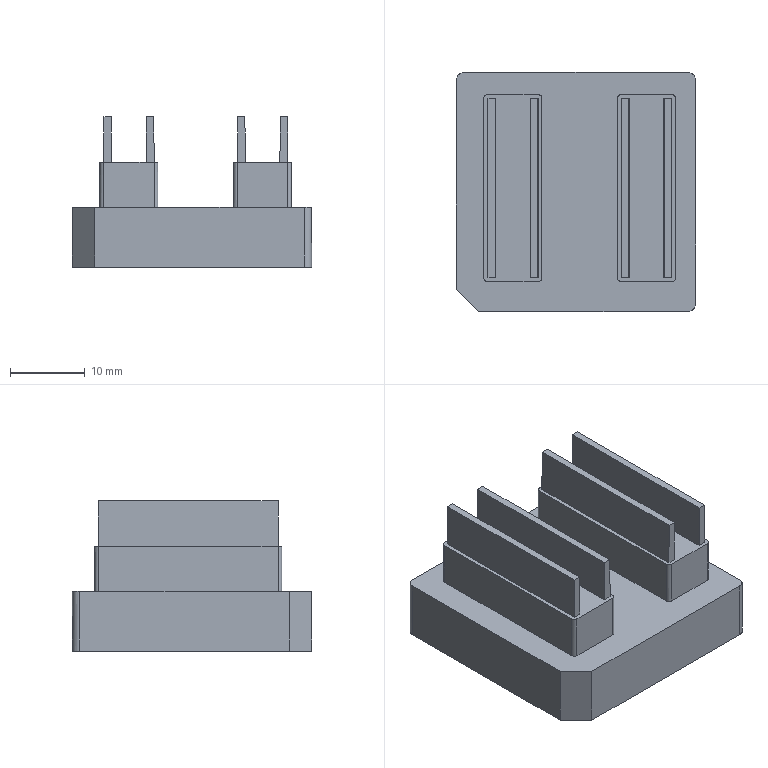NC program | PowerMill | posted with a generic post | part box 32 x 32 x 20.109 mm
Lines 18577 to 19554 of 124326:
N18674 M6
N18675 S18000 M03
N18676 G00 G90 X0.0 Y0.0
N18677 G43 Z10.799 H10
N18678
N18679 G05 P10000 R8
N18680 X9.9087 Y3.019
N18681 Z0.909
N18682 G01 Z-0.291 F1200.0
N18683 X9.9524 Y3.021 F2000.0
N18684 X9.9957 Y3.0269
N18685 X10.0383 Y3.0368
N18686 X10.0799 Y3.0506
N18687 X10.12 Y3.068
N18688 X10.1584 Y3.0891
N18689 X10.1947 Y3.1135
N18690 X10.2286 Y3.1412
N18691 X10.2599 Y3.1718
N18692 X10.2882 Y3.2051
N18693 X10.3134 Y3.2409
N18694 X10.3352 Y3.2788
N18695 X10.3535 Y3.3186
N18696 X10.3681 Y3.3599
N18697 X10.3788 Y3.4023
N18698 X10.3857 Y3.4455
N18699 X10.3886 Y3.4891
N18700 X10.3887 Y3.499
N18701 Y9.4972
N18702 X10.3886 Y11.6966
N18703 X10.3881 Y12.4964
N18704 X10.39 Y12.5743
N18705 X10.3958 Y12.6519
N18706 X10.4056 Y12.7286
N18707 X10.4192 Y12.8042
N18708 X10.4365 Y12.8783
N18709 X10.4575 Y12.9506
N18710 X10.482 Y13.0208
N18711 X10.5098 Y13.0888
N18712 X10.5412 Y13.1551
N18713 X10.5769 Y13.2214
N18714 X10.616 Y13.2858
N18715 X10.6586 Y13.3481
N18716 X10.7044 Y13.408
N18717 X10.7533 Y13.4655
N18718 X10.8052 Y13.5203
N18719 X10.8599 Y13.5723
N18720 X10.9172 Y13.6212
N18721 X10.9769 Y13.667
N18722 X11.039 Y13.7095
N18723 X11.1032 Y13.7487
N18724 X11.1695 Y13.7845
N18725 X11.2373 Y13.8166
N18726 X11.3079 Y13.8456
N18727 X11.3794 Y13.8707
N18728 X11.4516 Y13.8919
N18729 X11.5242 Y13.9091
N18730 X11.5972 Y13.9222
N18731 X11.6701 Y13.9314
N18732 X11.7429 Y13.9366
N18733 X11.8156 Y13.9379
N18734 X12.5481 Y13.9385
N18735 X12.7962 Y13.9378
N18736 X12.8681 Y13.9356
N18737 X12.9404 Y13.9294
N18738 X13.0129 Y13.9191
N18739 X13.0856 Y13.9048
N18740 X13.1581 Y13.8865
N18741 X13.2303 Y13.8642
N18742 X13.3019 Y13.8379
N18743 X13.3726 Y13.8077
N18744 X13.4395 Y13.7749
N18745 X13.5046 Y13.7386
N18746 X13.568 Y13.6987
N18747 X13.6293 Y13.6554
N18748 X13.6884 Y13.6087
N18749 X13.7452 Y13.5589
N18750 X13.7987 Y13.5066
N18751 X13.8494 Y13.4516
N18752 X13.8973 Y13.3938
N18753 X13.9422 Y13.3333
N18754 X13.984 Y13.2702
N18755 X14.0227 Y13.2048
N18756 X14.058 Y13.137
N18757 X14.0899 Y13.0672
N18758 X14.1164 Y13.0003
N18759 X14.1393 Y12.9316
N18760 X14.1588 Y12.8606
N18761 X14.1748 Y12.7875
N18762 X14.1872 Y12.7125
N18763 X14.1958 Y12.6355
N18764 X14.2007 Y12.5567
N18765 X14.2018 Y12.4763
N18766 Y-1.4479
N18767 Y-9.9971
N18768 X14.2017 Y-11.0461
N18769 X14.2022 Y-11.4967
N18770 X14.2004 Y-11.5753
N18771 X14.1946 Y-11.6529
N18772 X14.1851 Y-11.7293
N18773 X14.1717 Y-11.804
N18774 X14.1547 Y-11.8769
N18775 X14.1341 Y-11.9478
N18776 X14.1101 Y-12.0169
N18777 X14.0815 Y-12.0865
N18778 X14.0494 Y-12.1546
N18779 X14.0137 Y-12.221
N18780 X13.9746 Y-12.2853
N18781 X13.9321 Y-12.3476
N18782 X13.8863 Y-12.4076
N18783 X13.8374 Y-12.4651
N18784 X13.7855 Y-12.5199
N18785 X13.7308 Y-12.5719
N18786 X13.6734 Y-12.621
N18787 X13.6136 Y-12.6668
N18788 X13.5515 Y-12.7094
N18789 X13.4873 Y-12.7487
N18790 X13.4211 Y-12.7844
N18791 X13.3532 Y-12.8166
N18792 X13.2838 Y-12.8452
N18793 X13.213 Y-12.87
N18794 X13.1409 Y-12.8911
N18795 X13.1212 Y-12.8961
N18796 X13.047 Y-12.9127
N18797 X12.9737 Y-12.925
N18798 X12.9016 Y-12.9332
N18799 X12.8308 Y-12.9375
N18800 X12.7606 Y-12.9382
N18801 X12.2312 Y-12.9385
N18802 X11.7966 Y-12.9378
N18803 X11.724 Y-12.9358
N18804 X11.6514 Y-12.9297
N18805 X11.5788 Y-12.9197
N18806 X11.5064 Y-12.9057
N18807 X11.4343 Y-12.8877
N18808 X11.3628 Y-12.8657
N18809 X11.2921 Y-12.8398
N18810 X11.2224 Y-12.81
N18811 X11.154 Y-12.7764
N18812 X11.0871 Y-12.7391
N18813 X11.0219 Y-12.6983
N18814 X10.962 Y-12.6561
N18815 X10.9038 Y-12.6103
N18816 X10.8474 Y-12.5609
N18817 X10.7935 Y-12.5085
N18818 X10.7425 Y-12.4533
N18819 X10.6944 Y-12.3954
N18820 X10.6494 Y-12.335
N18821 X10.6075 Y-12.2721
N18822 X10.5689 Y-12.207
N18823 X10.5337 Y-12.1397
N18824 X10.502 Y-12.0705
N18825 X10.4739 Y-11.9996
N18826 X10.451 Y-11.9314
N18827 X10.4316 Y-11.8612
N18828 X10.4157 Y-11.7888
N18829 X10.4034 Y-11.7142
N18830 X10.3947 Y-11.6375
N18831 X10.3898 Y-11.5587
N18832 X10.3887 Y-11.4781
N18833 Y3.499
N18834 X10.3867 Y3.5427
N18835 X10.3807 Y3.586
N18836 X10.3708 Y3.6287
N18837 X10.3571 Y3.6702
N18838 X10.3396 Y3.7104
N18839 X10.3186 Y3.7487
N18840 X10.2941 Y3.785
N18841 X10.2665 Y3.8189
N18842 X10.2359 Y3.8502
N18843 X10.2025 Y3.8785
N18844 X10.1668 Y3.9037
N18845 X10.1288 Y3.9255
N18846 X10.089 Y3.9438
N18847 X10.0478 Y3.9584
N18848 X10.0054 Y3.9691
N18849 X9.9622 Y3.976
N18850 X9.9185 Y3.9789
N18851 X9.9087 Y3.979
N18852 X9.9083 Y3.019 Z-0.331
N18853 X9.952 Y3.021
N18854 X9.9953 Y3.0269
N18855 X10.038 Y3.0368
N18856 X10.0795 Y3.0506
N18857 X10.1197 Y3.068
N18858 X10.158 Y3.0891
N18859 X10.1943 Y3.1135
N18860 X10.2282 Y3.1412
N18861 X10.2595 Y3.1718
N18862 X10.2878 Y3.2051
N18863 X10.313 Y3.2409
N18864 X10.3348 Y3.2788
N18865 X10.3531 Y3.3186
N18866 X10.3677 Y3.3599
N18867 X10.3784 Y3.4023
N18868 X10.3853 Y3.4455
N18869 X10.3882 Y3.4891
N18870 X10.3883 Y3.499
N18871 Y10.9968
N18872 Y12.4963
N18873 X10.3902 Y12.5756
N18874 X10.396 Y12.6536
N18875 X10.4057 Y12.7303
N18876 X10.4191 Y12.8053
N18877 X10.4362 Y12.8786
N18878 X10.4569 Y12.9499
N18879 X10.481 Y13.0192
N18880 X10.5087 Y13.0866
N18881 X10.541 Y13.1551
N18882 X10.577 Y13.2218
N18883 X10.6163 Y13.2865
N18884 X10.659 Y13.349
N18885 X10.7049 Y13.409
N18886 X10.7538 Y13.4664
N18887 X10.8056 Y13.5211
N18888 X10.8601 Y13.5729
N18889 X10.9173 Y13.6217
N18890 X10.9769 Y13.6674
N18891 X11.0388 Y13.7097
N18892 X11.1033 Y13.7491
N18893 X11.1698 Y13.785
N18894 X11.238 Y13.8173
N18895 X11.3078 Y13.8459
N18896 X11.3788 Y13.8708
N18897 X11.451 Y13.8918
N18898 X11.524 Y13.9089
N18899 X11.5976 Y13.9221
N18900 X11.6718 Y13.9313
N18901 X11.7463 Y13.9365
N18902 X11.821 Y13.938
N18903 X12.1312 Y13.9386
N18904 X12.665 Y13.9382
N18905 X12.7963 Y13.9378
N18906 X12.8692 Y13.9355
N18907 X12.9421 Y13.9292
N18908 X13.0151 Y13.9189
N18909 X13.0878 Y13.9046
N18910 X13.1602 Y13.8864
N18911 X13.232 Y13.8642
N18912 X13.303 Y13.838
N18913 X13.373 Y13.808
N18914 X13.4403 Y13.7748
N18915 X13.5058 Y13.7381
N18916 X13.5694 Y13.698
N18917 X13.6309 Y13.6544
N18918 X13.69 Y13.6076
N18919 X13.7468 Y13.5576
N18920 X13.8008 Y13.5047
N18921 X13.8521 Y13.4489
N18922 X13.8991 Y13.392
N18923 X13.9431 Y13.3327
N18924 X13.9843 Y13.2705
N18925 X14.0226 Y13.2055
N18926 X14.058 Y13.1377
N18927 X14.0902 Y13.0671
N18928 X14.1167 Y13.0006
N18929 X14.1396 Y12.9322
N18930 X14.159 Y12.8615
N18931 X14.175 Y12.7887
N18932 X14.1874 Y12.7138
N18933 X14.1961 Y12.6369
N18934 X14.201 Y12.5581
N18935 X14.2021 Y12.4776
N18936 Y-1.9367
N18937 Y-9.9971
N18938 Y-11.4966
N18939 X14.2002 Y-11.5768
N18940 X14.1945 Y-11.655
N18941 X14.185 Y-11.7311
N18942 X14.1719 Y-11.8051
N18943 X14.1552 Y-11.8768
N18944 X14.1351 Y-11.9463
N18945 X14.1114 Y-12.014
N18946 X14.0823 Y-12.0853
N18947 X14.0498 Y-12.1543
N18948 X14.0141 Y-12.2209
N18949 X13.9753 Y-12.285
N18950 X13.9335 Y-12.3464
N18951 X13.8886 Y-12.4052
N18952 X13.8396 Y-12.4629
N18953 X13.7876 Y-12.518
N18954 X13.7329 Y-12.5702
N18955 X13.6755 Y-12.6194
N18956 X13.6156 Y-12.6655
N18957 X13.5535 Y-12.7083
N18958 X13.4892 Y-12.7476
N18959 X13.4231 Y-12.7835
N18960 X13.3552 Y-12.8158
N18961 X13.2858 Y-12.8444
N18962 X13.215 Y-12.8693
N18963 X13.143 Y-12.8904
N18964 X13.1215 Y-12.8958
N18965 X13.1212 Y-12.8959
N18966 X13.0454 Y-12.9128
N18967 X12.9721 Y-12.9252
N18968 X12.9015 Y-12.9335
N18969 X12.8332 Y-12.9376
N18970 X12.7662 Y-12.9383
N18971 X12.2196 Y-12.9387
N18972 X11.7966 Y-12.938
N18973 X11.7238 Y-12.9357
N18974 X11.6508 Y-12.9294
N18975 X11.5777 Y-12.9191
N18976 X11.5047 Y-12.9049
N18977 X11.432 Y-12.8866
N18978 X11.3598 Y-12.8643
N18979 X11.2884 Y-12.8381
N18980 X11.2181 Y-12.8081
N18981 X11.151 Y-12.7752
N18982 X11.0856 Y-12.7388
N18983 X11.0222 Y-12.6988
N18984 X10.9608 Y-12.6554
N18985 X10.9016 Y-12.6088
N18986 X10.8449 Y-12.5589
N18987 X10.7912 Y-12.5065
N18988 X10.7404 Y-12.4512
N18989 X10.6924 Y-12.3933
N18990 X10.6474 Y-12.3327
N18991 X10.6056 Y-12.2695
N18992 X10.5669 Y-12.204
N18993 X10.5315 Y-12.1362
N18994 X10.5011 Y-12.0699
N18995 X10.4744 Y-12.0022
N18996 X10.4511 Y-11.9326
N18997 X10.4315 Y-11.8611
N18998 X10.4154 Y-11.7878
N18999 X10.403 Y-11.7126
N19000 X10.3943 Y-11.6357
N19001 X10.3894 Y-11.5571
N19002 X10.3883 Y-11.477
N19003 Y1.9985
N19004 Y3.499
N19005 X10.3863 Y3.5427
N19006 X10.3803 Y3.586
N19007 X10.3704 Y3.6287
N19008 X10.3567 Y3.6702
N19009 X10.3392 Y3.7104
N19010 X10.3182 Y3.7487
N19011 X10.2937 Y3.785
N19012 X10.2661 Y3.8189
N19013 X10.2355 Y3.8502
N19014 X10.2021 Y3.8785
N19015 X10.1664 Y3.9037
N19016 X10.1284 Y3.9255
N19017 X10.0887 Y3.9438
N19018 X10.0474 Y3.9584
N19019 X10.005 Y3.9691
N19020 X9.9618 Y3.976
N19021 X9.9181 Y3.9789
N19022 X9.9083 Y3.979
N19023 X9.9079 Y3.019 Z-0.371
N19024 X9.9516 Y3.021
N19025 X9.995 Y3.0269
N19026 X10.0376 Y3.0368
N19027 X10.0792 Y3.0506
N19028 X10.1193 Y3.068
N19029 X10.1577 Y3.0891
N19030 X10.194 Y3.1135
N19031 X10.2279 Y3.1412
N19032 X10.2591 Y3.1718
N19033 X10.2875 Y3.2051
N19034 X10.3126 Y3.2409
N19035 X10.3345 Y3.2788
N19036 X10.3527 Y3.3186
N19037 X10.3673 Y3.3599
N19038 X10.3781 Y3.4023
N19039 X10.3849 Y3.4455
N19040 X10.3878 Y3.4891
N19041 X10.3879 Y3.499
N19042 Y5.089
N19043 Y12.4963
N19044 X10.3896 Y12.5773
N19045 X10.3946 Y12.6507
N19046 X10.403 Y12.7203
N19047 X10.4159 Y12.7945
N19048 X10.4327 Y12.8679
N19049 X10.4534 Y12.9404
N19050 X10.4779 Y13.0117
N19051 X10.5061 Y13.0817
N19052 X10.538 Y13.1501
N19053 X10.5735 Y13.2167
N19054 X10.6124 Y13.2813
N19055 X10.6547 Y13.3437
N19056 X10.7002 Y13.4038
N19057 X10.7488 Y13.4613
N19058 X10.8003 Y13.5162
N19059 X10.8547 Y13.5683
N19060 X10.9117 Y13.6173
N19061 X10.9715 Y13.6636
N19062 X11.0331 Y13.7062
N19063 X11.0962 Y13.7452
N19064 X11.1608 Y13.7804
N19065 X11.2269 Y13.812
N19066 X11.2988 Y13.842
N19067 X11.3711 Y13.868
N19068 X11.4437 Y13.8899
N19069 X11.5161 Y13.9077
N19070 X11.5884 Y13.9214
N19071 X11.6602 Y13.9311
N19072 X11.7315 Y13.9367
N19073 X11.8023 Y13.9384
N19074 X12.2964
N19075 X12.662
N19076 X12.7963 Y13.9378
N19077 X12.8703 Y13.9352
N19078 X12.9442 Y13.9287
N19079 X13.0179 Y13.9182
N19080 X13.0912 Y13.9037
N19081 X13.1638 Y13.8852
N19082 X13.2357 Y13.8629
N19083 X13.3066 Y13.8367
N19084 X13.3762 Y13.8066
N19085 X13.4434 Y13.7734
N19086 X13.5089 Y13.7365
N19087 X13.5724 Y13.6962
N19088 X13.6339 Y13.6524
N19089 X13.6931 Y13.6054
N19090 X13.7498 Y13.5551
N19091 X13.803 Y13.5029
N19092 X13.8534 Y13.4479
N19093 X13.9009 Y13.3901
N19094 X13.9455 Y13.3296
N19095 X13.9872 Y13.2664
N19096 X14.0257 Y13.2007
N19097 X14.0609 Y13.1326
N19098 X14.0911 Y13.0663
N19099 X14.1177 Y12.9985
N19100 X14.1407 Y12.929
N19101 X14.1602 Y12.8574
N19102 X14.1761 Y12.784
N19103 X14.1883 Y12.7088
N19104 X14.1968 Y12.6318
N19105 X14.2015 Y12.5531
N19106 X14.2025 Y12.4728
N19107 Y-0.872
N19108 Y-8.6378
N19109 X14.2026 Y-10.7936
N19110 X14.2028 Y-11.4966
N19111 X14.2009 Y-11.5762
N19112 X14.1952 Y-11.6541
N19113 X14.1857 Y-11.7302
N19114 X14.1725 Y-11.8043
N19115 X14.1557 Y-11.8763
N19116 X14.1354 Y-11.9462
N19117 X14.1116 Y-12.0143
N19118 X14.0823 Y-12.0858
N19119 X14.0499 Y-12.1549
N19120 X14.0144 Y-12.2212
N19121 X13.9758 Y-12.2849
N19122 X13.9345 Y-12.3456
N19123 X13.8902 Y-12.4036
N19124 X13.8402 Y-12.4626
N19125 X13.7886 Y-12.5176
N19126 X13.7352 Y-12.5687
N19127 X13.6796 Y-12.6167
N19128 X13.6197 Y-12.663
N19129 X13.5576 Y-12.706
N19130 X13.4935 Y-12.7456
N19131 X13.4274 Y-12.7817
N19132 X13.3597 Y-12.8142
N19133 X13.2904 Y-12.8429
N19134 X13.2197 Y-12.868
N19135 X13.1478 Y-12.8892
N19136 X13.1219 Y-12.8959
N19137 X13.1212 Y-12.896
N19138 X13.0456 Y-12.9128
N19139 X12.9721 Y-12.9253
N19140 X12.9014 Y-12.9335
N19141 X12.8331 Y-12.9376
N19142 X12.766 Y-12.9383
N19143 X12.2057 Y-12.9387
N19144 X11.7966 Y-12.9379
N19145 X11.7236 Y-12.9357
N19146 X11.6505 Y-12.9294
N19147 X11.5773 Y-12.9191
N19148 X11.5043 Y-12.9048
N19149 X11.4316 Y-12.8866
N19150 X11.3595 Y-12.8644
N19151 X11.2882 Y-12.8382
N19152 X11.218 Y-12.8082
N19153 X11.1506 Y-12.7752
N19154 X11.0851 Y-12.7386
N19155 X11.0215 Y-12.6986
N19156 X10.9601 Y-12.6552
N19157 X10.9009 Y-12.6085
N19158 X10.8443 Y-12.5587
N19159 X10.7903 Y-12.506
N19160 X10.7393 Y-12.4505
N19161 X10.6915 Y-12.3927
N19162 X10.6469 Y-12.3325
N19163 X10.6053 Y-12.2699
N19164 X10.567 Y-12.2048
N19165 X10.5319 Y-12.1373
N19166 X10.5001 Y-12.0677
N19167 X10.472 Y-11.9965
N19168 X10.4494 Y-11.9288
N19169 X10.4302 Y-11.859
N19170 X10.4145 Y-11.7868
N19171 X10.4023 Y-11.7124
N19172 X10.3938 Y-11.6357
N19173 X10.389 Y-11.5569
N19174 X10.3879 Y-11.476
N19175 Y3.499
N19176 X10.3859 Y3.5427
N19177 X10.38 Y3.586
N19178 X10.3701 Y3.6287
N19179 X10.3563 Y3.6702
N19180 X10.3389 Y3.7104
N19181 X10.3178 Y3.7487
N19182 X10.2934 Y3.785
N19183 X10.2657 Y3.8189
N19184 X10.2351 Y3.8502
N19185 X10.2018 Y3.8785
N19186 X10.166 Y3.9037
N19187 X10.1281 Y3.9255
N19188 X10.0883 Y3.9438
N19189 X10.0471 Y3.9584
N19190 X10.0046 Y3.9691
N19191 X9.9614 Y3.976
N19192 X9.9178 Y3.9789
N19193 X9.9079 Y3.979
N19194 X9.9076 Y3.019 Z-0.411
N19195 X9.9513 Y3.021
N19196 X9.9946 Y3.0269
N19197 X10.0373 Y3.0368
N19198 X10.0788 Y3.0506
N19199 X10.119 Y3.068
N19200 X10.1573 Y3.0891
N19201 X10.1936 Y3.1135
N19202 X10.2275 Y3.1412
N19203 X10.2588 Y3.1718
N19204 X10.2871 Y3.2051
N19205 X10.3123 Y3.2409
N19206 X10.3341 Y3.2788
N19207 X10.3524 Y3.3186
N19208 X10.367 Y3.3599
N19209 X10.3777 Y3.4023
N19210 X10.3846 Y3.4455
N19211 X10.3875 Y3.4891
N19212 X10.3876 Y3.499
N19213 Y5.1533
N19214 Y12.4963
N19215 X10.3893 Y12.5773
N19216 X10.3943 Y12.6512
N19217 X10.4028 Y12.7213
N19218 X10.4158 Y12.7956
N19219 X10.4326 Y12.8691
N19220 X10.4534 Y12.9415
N19221 X10.4779 Y13.0128
N19222 X10.5062 Y13.0827
N19223 X10.5381 Y13.1511
N19224 X10.5737 Y13.2176
N19225 X10.6127 Y13.2822
N19226 X10.655 Y13.3446
N19227 X10.7006 Y13.4046
N19228 X10.7493 Y13.4622
N19229 X10.8009 Y13.5171
N19230 X10.8554 Y13.5691
N19231 X10.9124 Y13.6181
N19232 X10.9723 Y13.6643
N19233 X11.0345 Y13.7072
N19234 X11.0989 Y13.7468
N19235 X11.1652 Y13.783
N19236 X11.2333 Y13.8155
N19237 X11.3029 Y13.8444
N19238 X11.3738 Y13.8694
N19239 X11.4457 Y13.8907
N19240 X11.5185 Y13.908
N19241 X11.5919 Y13.9214
N19242 X11.6658 Y13.9308
N19243 X11.74 Y13.9363
N19244 X11.8144 Y13.9378
N19245 X12.2538 Y13.9388
N19246 X12.6931 Y13.9381
N19247 X12.7959 Y13.938
N19248 X12.8664 Y13.936
N19249 X12.9379 Y13.93
N19250 X13.0102 Y13.9199
N19251 X13.083 Y13.9058
N19252 X13.1558 Y13.8875
N19253 X13.2284 Y13.8653
N19254 X13.3001 Y13.8392
N19255 X13.3706 Y13.8093
N19256 X13.4369 Y13.777
N19257 X13.5017 Y13.7411
N19258 X13.5651 Y13.7013
N19259 X13.6267 Y13.658
N19260 X13.6863 Y13.6113
N19261 X13.7434 Y13.5614
N19262 X13.7978 Y13.5086
N19263 X13.8491 Y13.4531
N19264 X13.8973 Y13.3954
N19265 X13.942 Y13.3355
N19266 X13.9832 Y13.2737
N19267 X14.0213 Y13.2095
N19268 X14.0563 Y13.1424
N19269 X14.0884 Y13.0727
N19270 X14.1172 Y13.0004
N19271 X14.14 Y12.9332
N19272 X14.1594 Y12.8638
N19273 X14.1753 Y12.7921
N19274 X14.1877 Y12.718
N19275 X14.1965 Y12.6416
N19276 X14.2015 Y12.5629
N19277 X14.2028 Y12.4819
N19278 Y-2.4993
N19279 Y-8.4975
N19280 X14.2029 Y-10.6969
N19281 X14.2033 Y-11.4967
N19282 X14.2014 Y-11.5747
N19283 X14.1956 Y-11.652
N19284 X14.1859 Y-11.7284
N19285 X14.1723 Y-11.8037
N19286 X14.1549 Y-11.8777
N19287 X14.1338 Y-11.9503
N19288 X14.109 Y-12.0214
N19289 X14.0806 Y-12.0908
N19290 X14.0486 Y-12.1583
N19291 X14.0131 Y-12.224
N19292 X13.9742 Y-12.2878
N19293 X13.9316 Y-12.3499
N19294 X13.8858 Y-12.4096
N19295 X13.837 Y-12.4669
N19296 X13.7851 Y-12.5215
N19297 X13.7304 Y-12.5734
N19298 X13.673 Y-12.6223
N19299 X13.6131 Y-12.668
N19300 X13.5509 Y-12.7106
N19301 X13.4866 Y-12.7497
N19302 X13.4203 Y-12.7854
N19303 X13.3523 Y-12.8174
N19304 X13.2827 Y-12.8459
N19305 X13.2116 Y-12.8706
N19306 X13.1394 Y-12.8915
N19307 X13.1222 Y-12.8958
N19308 X13.1212 Y-12.8961
N19309 X13.0463 Y-12.9127
N19310 X12.973 Y-12.9252
N19311 X12.9022 Y-12.9335
N19312 X12.8337 Y-12.9376
N19313 X12.7664 Y-12.9383
N19314 X12.1869 Y-12.9387
N19315 X11.7966 Y-12.938
N19316 X11.7236 Y-12.9357
N19317 X11.6504 Y-12.9294
N19318 X11.5772 Y-12.9191
N19319 X11.5041 Y-12.9049
N19320 X11.4314 Y-12.8866
N19321 X11.3593 Y-12.8644
N19322 X11.288 Y-12.8383
N19323 X11.2178 Y-12.8083
N19324 X11.1505 Y-12.7753
N19325 X11.0849 Y-12.7387
N19326 X11.0213 Y-12.6987
N19327 X10.9599 Y-12.6553
N19328 X10.9007 Y-12.6086
N19329 X10.8441 Y-12.5588
N19330 X10.7901 Y-12.5061
N19331 X10.739 Y-12.4506
N19332 X10.6913 Y-12.3929
N19333 X10.6466 Y-12.3327
N19334 X10.6051 Y-12.27
N19335 X10.5667 Y-12.2049
N19336 X10.5316 Y-12.1375
N19337 X10.4999 Y-12.0679
N19338 X10.4717 Y-11.9965
N19339 X10.449 Y-11.9288
N19340 X10.4299 Y-11.859
N19341 X10.4141 Y-11.7868
N19342 X10.402 Y-11.7124
N19343 X10.3934 Y-11.6358
N19344 X10.3887 Y-11.5569
N19345 X10.3876 Y-11.476
N19346 Y3.499
N19347 X10.3856 Y3.5427
N19348 X10.3796 Y3.586
N19349 X10.3697 Y3.6287
N19350 X10.356 Y3.6702
N19351 X10.3385 Y3.7104
N19352 X10.3175 Y3.7487
N19353 X10.293 Y3.785
N19354 X10.2654 Y3.8189
N19355 X10.2348 Y3.8502
N19356 X10.2014 Y3.8785
N19357 X10.1657 Y3.9037
N19358 X10.1277 Y3.9255
N19359 X10.088 Y3.9438
N19360 X10.0467 Y3.9584
N19361 X10.0043 Y3.9691
N19362 X9.9611 Y3.976
N19363 X9.9174 Y3.9789
N19364 X9.9076 Y3.979
N19365 X9.9072 Y3.019 Z-0.451
N19366 X9.9509 Y3.021
N19367 X9.9943 Y3.0269
N19368 X10.0369 Y3.0368
N19369 X10.0785 Y3.0506
N19370 X10.1186 Y3.068
N19371 X10.157 Y3.0891
N19372 X10.1933 Y3.1135
N19373 X10.2272 Y3.1412
N19374 X10.2584 Y3.1718
N19375 X10.2868 Y3.2051
N19376 X10.3119 Y3.2409
N19377 X10.3338 Y3.2788
N19378 X10.352 Y3.3186
N19379 X10.3666 Y3.3599
N19380 X10.3774 Y3.4023
N19381 X10.3842 Y3.4455
N19382 X10.3871 Y3.4891
N19383 X10.3872 Y3.499
N19384 Y10.9968
N19385 Y12.4963
N19386 X10.3892 Y12.5755
N19387 X10.395 Y12.6536
N19388 X10.4047 Y12.7303
N19389 X10.4181 Y12.8053
N19390 X10.4352 Y12.8786
N19391 X10.4559 Y12.95
N19392 X10.48 Y13.0193
N19393 X10.5077 Y13.0868
N19394 X10.5401 Y13.1553
N19395 X10.576 Y13.222
N19396 X10.6154 Y13.2866
N19397 X10.6581 Y13.3491
N19398 X10.7039 Y13.4091
N19399 X10.7528 Y13.4665
N19400 X10.8046 Y13.5212
N19401 X10.8592 Y13.573
N19402 X10.9164 Y13.6218
N19403 X10.9761 Y13.6675
N19404 X11.0379 Y13.7098
N19405 X11.1024 Y13.7492
N19406 X11.1689 Y13.7851
N19407 X11.2371 Y13.8174
N19408 X11.3069 Y13.846
N19409 X11.378 Y13.8708
N19410 X11.4501 Y13.8918
N19411 X11.5232 Y13.9089
N19412 X11.5969 Y13.9221
N19413 X11.6711 Y13.9313
N19414 X11.7456 Y13.9366
N19415 X11.8204 Y13.938
N19416 X12.1406 Y13.9386
N19417 X12.6911 Y13.9381
N19418 X12.7963 Y13.9378
N19419 X12.8693 Y13.9355
N19420 X12.9424 Y13.9293
N19421 X13.0154 Y13.919
N19422 X13.0883 Y13.9048
N19423 X13.1607 Y13.8865
N19424 X13.2325 Y13.8643
N19425 X13.3035 Y13.8382
N19426 X13.3735 Y13.8082
N19427 X13.4408 Y13.7751
N19428 X13.5064 Y13.7385
N19429 X13.5699 Y13.6983
N19430 X13.6314 Y13.6548
N19431 X13.6906 Y13.608
N19432 X13.7474 Y13.5581
N19433 X13.8015 Y13.5051
N19434 X13.8527 Y13.4493
N19435 X13.9001 Y13.3921
N19436 X13.9443 Y13.3325
N19437 X13.9856 Y13.2702
N19438 X14.0238 Y13.2054
N19439 X14.0589 Y13.138
N19440 X14.0907 Y13.0683
N19441 X14.1191 Y12.9964
N19442 X14.1417 Y12.9288
N19443 X14.1609 Y12.8591
N19444 X14.1766 Y12.7871
N19445 X14.1887 Y12.7127
N19446 X14.1973 Y12.6361
N19447 X14.2021 Y12.5572
N19448 X14.2032 Y12.4761
N19449 Y-3.7798
N19450 Y-9.9971
N19451 Y-11.4966
N19452 X14.2013 Y-11.5768
N19453 X14.1955 Y-11.655
N19454 X14.186 Y-11.7311
N19455 X14.1729 Y-11.8051
N19456 X14.1563 Y-11.8768
N19457 X14.1361 Y-11.9463
N19458 X14.1125 Y-12.0139
N19459 X14.0833 Y-12.0852
N19460 X14.0509 Y-12.1543
N19461 X14.0152 Y-12.2209
N19462 X13.9763 Y-12.285
N19463 X13.9345 Y-12.3464
N19464 X13.8897 Y-12.4052
N19465 X13.8406 Y-12.4629
N19466 X13.7887 Y-12.518
N19467 X13.7339 Y-12.5702
N19468 X13.6765 Y-12.6194
N19469 X13.6167 Y-12.6655
N19470 X13.5545 Y-12.7082
N19471 X13.4903 Y-12.7476
N19472 X13.4241 Y-12.7835
N19473 X13.3563 Y-12.8158
N19474 X13.2868 Y-12.8444
N19475 X13.216 Y-12.8693
N19476 X13.144 Y-12.8904
N19477 X13.1226 Y-12.8959
N19478 X13.1212 Y-12.8962
N19479 X13.0466 Y-12.9127
N19480 X12.9733 Y-12.9252
N19481 X12.9024 Y-12.9335
N19482 X12.8337 Y-12.9376
N19483 X12.7662 Y-12.9383
N19484 X12.1582 Y-12.9386
N19485 X11.7966 Y-12.938
N19486 X11.7236 Y-12.9357
N19487 X11.6506 Y-12.9295
N19488 X11.5774 Y-12.9192
N19489 X11.5043 Y-12.905
N19490 X11.4315 Y-12.8867
N19491 X11.3594 Y-12.8645
N19492 X11.288 Y-12.8384
N19493 X11.2176 Y-12.8084
N19494 X11.1505 Y-12.7755
N19495 X11.0851 Y-12.7391
N19496 X11.0216 Y-12.6991
N19497 X10.9601 Y-12.6558
N19498 X10.901 Y-12.6091
N19499 X10.8442 Y-12.5593
N19500 X10.7906 Y-12.5069
N19501 X10.7397 Y-12.4516
N19502 X10.6917 Y-12.3937
N19503 X10.6467 Y-12.3331
N19504 X10.6048 Y-12.27
N19505 X10.5661 Y-12.2045
N19506 X10.5307 Y-12.1367
N19507 X10.5003 Y-12.0704
N19508 X10.4735 Y-12.0027
N19509 X10.4503 Y-11.9331
N19510 X10.4305 Y-11.8617
N19511 X10.4144 Y-11.7883
N19512 X10.402 Y-11.7132
N19513 X10.3933 Y-11.6363
N19514 X10.3884 Y-11.5577
N19515 X10.3872 Y-11.4776
N19516 Y2.0884
N19517 Y3.499
N19518 X10.3852 Y3.5427
N19519 X10.3793 Y3.586
N19520 X10.3694 Y3.6287
N19521 X10.3556 Y3.6702
N19522 X10.3382 Y3.7104
N19523 X10.3171 Y3.7487
N19524 X10.2927 Y3.785
N19525 X10.265 Y3.8189
N19526 X10.2344 Y3.8502
N19527 X10.2011 Y3.8785
N19528 X10.1653 Y3.9037
N19529 X10.1274 Y3.9255
N19530 X10.0876 Y3.9438
N19531 X10.0464 Y3.9584
N19532 X10.0039 Y3.9691
N19533 X9.9607 Y3.976
N19534 X9.9171 Y3.9789
N19535 X9.9072 Y3.979
N19536 X9.9069 Y3.019 Z-0.491
N19537 X9.9506 Y3.021
N19538 X9.9939 Y3.0269
N19539 X10.0366 Y3.0368
N19540 X10.0781 Y3.0506
N19541 X10.1183 Y3.068
N19542 X10.1566 Y3.0891
N19543 X10.1929 Y3.1135
N19544 X10.2268 Y3.1412
N19545 X10.2581 Y3.1718
N19546 X10.2864 Y3.2051
N19547 X10.3116 Y3.2409
N19548 X10.3334 Y3.2788
N19549 X10.3517 Y3.3186
N19550 X10.3663 Y3.3599
N19551 X10.377 Y3.4023
N19552 X10.3839 Y3.4455
N19553 X10.3868 Y3.4891
N19554 X10.3869 Y3.499
N19555 Y8.6459
N19556 Y10.9968
N19557 Y12.4963
N19558 X10.3888 Y12.5754
N19559 X10.3947 Y12.6534
N19560 X10.4044 Y12.7301
N19561 X10.4179 Y12.8053
N19562 X10.435 Y12.8789
N19563 X10.4558 Y12.9506
N19564 X10.4801 Y13.0204
N19565 X10.5078 Y13.0881
N19566 X10.5391 Y13.1542
N19567 X10.5748 Y13.2206
N19568 X10.6139 Y13.285
N19569 X10.6563 Y13.3472
N19570 X10.702 Y13.4071
N19571 X10.7507 Y13.4645
N19572 X10.8024 Y13.5193
N19573 X10.8569 Y13.5712
N19574 X10.9142 Y13.6202
N19575 X10.974 Y13.6662
N19576 X11.0361 Y13.7089
N19577 X11.1004 Y13.7482
N19578 X11.1666 Y13.784
N19579 X11.2346 Y13.8163
N19580 X11.3043 Y13.845
N19581 X11.3753 Y13.8699
N19582 X11.4477 Y13.8911
N19583 X11.5211 Y13.9085
N19584 X11.5949 Y13.9219
N19585 X11.6682 Y13.9313
N19586 X11.7411 Y13.9367
N19587 X11.8134 Y13.9382
N19588 X12.2245 Y13.9385
N19589 X12.7541 Y13.938
N19590 X12.8272 Y13.9373
N19591 X12.9003 Y13.9334
N19592 X12.9734 Y13.9254
N19593 X13.0464 Y13.9135
N19594 X13.1191 Y13.8976
N19595 X13.1913 Y13.8777
N19596 X13.2628 Y13.8538
N19597 X13.3334 Y13.8261
N19598 X13.4017 Y13.7951
N19599 X13.4684 Y13.7604
N19600 X13.5331 Y13.7223
N19601 X13.5959 Y13.6808
N19602 X13.6564 Y13.6359
N19603 X13.7147 Y13.5878
N19604 X13.7703 Y13.5366
N19605 X13.8233 Y13.4825
N19606 X13.8733 Y13.4256
N19607 X13.9194 Y13.3673
N19608 X13.9624 Y13.3066
N19609 X14.0024 Y13.2433
N19610 X14.0393 Y13.1773
N19611 X14.073 Y13.109
N19612 X14.1034 Y13.0383
N19613 X14.1282 Y12.9715
N19614 X14.1495 Y12.9033
N19615 X14.1674 Y12.8327
N19616 X14.1818 Y12.7598
N19617 X14.1927 Y12.6846
N19618 X14.1998 Y12.6071
N19619 X14.2032 Y12.5274
N19620 X14.2035 Y12.4456
N19621 Y-3.9483
N19622 Y-9.9971
N19623 Y-11.4966
N19624 X14.2016 Y-11.5775
N19625 X14.196 Y-11.6554
N19626 X14.1868 Y-11.7304
N19627 X14.1741 Y-11.8026
N19628 X14.1579 Y-11.8721
N19629 X14.1382 Y-11.9402
N19630 X14.1132 Y-12.0125
N19631 X14.0847 Y-12.0831
N19632 X14.0526 Y-12.1517
N19633 X14.0172 Y-12.2181
N19634 X13.9785 Y-12.2822
N19635 X13.9367 Y-12.3439
N19636 X13.8917 Y-12.4031
N19637 X13.8428 Y-12.4609
N19638 X13.7909 Y-12.5161
N19639 X13.7363 Y-12.5684
N19640 X13.679 Y-12.6177
N19641 X13.6192 Y-12.6639
N19642 X13.5571 Y-12.7068
N19643 X13.493 Y-12.7463
N19644 X13.4269 Y-12.7823
N19645 X13.3591 Y-12.8147
N19646 X13.2897 Y-12.8434
N19647 X13.219 Y-12.8684
N19648 X13.147 Y-12.8897
N19649 X13.1229 Y-12.8958
N19650 X13.1213 Y-12.8962
N19651 X13.0468 Y-12.9127